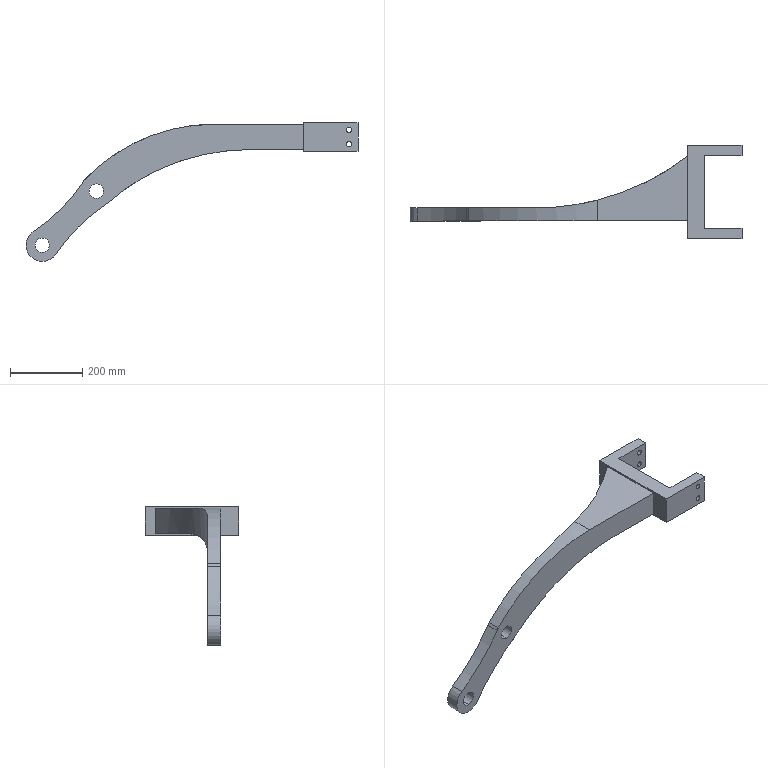Part | SolidWorks | features ICE 3, Cut 1, Extrusion 1 | 1 solid | 34 faces | box 920 x 260 x 385 mm | volume 5252996 mm3 | cylinder 20 | plane 14 | commonest cylinder face diameters 15 x8 40 x4 90 x3 1000 x2 984.464 x1 1199 x1
STEP:
#1=CARTESIAN_POINT('',(50.,-130.,-27.5));
#2=VERTEX_POINT('',#1);
#3=CARTESIAN_POINT('',(50.,-130.,-12.5));
#4=VERTEX_POINT('',#3);
#5=CARTESIAN_POINT('',(50.,-130.,-20.));
#6=DIRECTION('',(0.,1.,0.));
#7=DIRECTION('',(0.,0.,1.));
#8=AXIS2_PLACEMENT_3D('',#5,#6,#7);
#9=CIRCLE('',#8,7.5);
#10=EDGE_CURVE('',#2,#4,#9,.T.);
#11=ORIENTED_EDGE('',*,*,#10,.F.);
#12=CARTESIAN_POINT('',(50.,-100.,-27.5));
#13=VERTEX_POINT('',#12);
#14=CARTESIAN_POINT('',(50.,-130.,-27.5));
#15=DIRECTION('',(0.,1.,0.));
#16=VECTOR('',#15,1000.);
#17=LINE('',#14,#16);
#18=EDGE_CURVE('',#2,#13,#17,.T.);
#19=ORIENTED_EDGE('',*,*,#18,.T.);
#20=CARTESIAN_POINT('',(50.,-100.,-12.5));
#21=VERTEX_POINT('',#20);
#22=CARTESIAN_POINT('',(50.,-100.,-20.));
#23=DIRECTION('',(0.,-1.,0.));
#24=DIRECTION('',(0.,0.,-1.));
#25=AXIS2_PLACEMENT_3D('',#22,#23,#24);
#26=CIRCLE('',#25,7.5);
#27=EDGE_CURVE('',#21,#13,#26,.T.);
#28=ORIENTED_EDGE('',*,*,#27,.F.);
#29=CARTESIAN_POINT('',(50.,-130.,-12.5));
#30=DIRECTION('',(0.,1.,0.));
#31=VECTOR('',#30,1000.);
#32=LINE('',#29,#31);
#33=EDGE_CURVE('',#4,#21,#32,.T.);
#34=ORIENTED_EDGE('',*,*,#33,.F.);
#35=EDGE_LOOP('',(#11,#19,#28,#34));
#36=FACE_OUTER_BOUND('',#35,.T.);
#37=CARTESIAN_POINT('',(50.,-130.,-20.));
#38=DIRECTION('',(0.,1.,0.));
#39=DIRECTION('',(0.,0.,1.));
#40=AXIS2_PLACEMENT_3D('',#37,#38,#39);
#41=CYLINDRICAL_SURFACE('',#40,7.5);
#42=ADVANCED_FACE('',(#36),#41,.F.);
#43=CARTESIAN_POINT('',(50.,-130.,12.5));
#44=VERTEX_POINT('',#43);
#45=CARTESIAN_POINT('',(50.,-130.,27.5));
#46=VERTEX_POINT('',#45);
#47=CARTESIAN_POINT('',(50.,-130.,20.));
#48=DIRECTION('',(0.,1.,0.));
#49=DIRECTION('',(0.,0.,1.));
#50=AXIS2_PLACEMENT_3D('',#47,#48,#49);
#51=CIRCLE('',#50,7.5);
#52=EDGE_CURVE('',#44,#46,#51,.T.);
#53=ORIENTED_EDGE('',*,*,#52,.F.);
#54=CARTESIAN_POINT('',(50.,-100.,12.5));
#55=VERTEX_POINT('',#54);
#56=CARTESIAN_POINT('',(50.,-130.,12.5));
#57=DIRECTION('',(0.,1.,0.));
#58=VECTOR('',#57,1000.);
#59=LINE('',#56,#58);
#60=EDGE_CURVE('',#44,#55,#59,.T.);
#61=ORIENTED_EDGE('',*,*,#60,.T.);
#62=CARTESIAN_POINT('',(50.,-100.,27.5));
#63=VERTEX_POINT('',#62);
#64=CARTESIAN_POINT('',(50.,-100.,20.));
#65=DIRECTION('',(0.,-1.,0.));
#66=DIRECTION('',(0.,0.,-1.));
#67=AXIS2_PLACEMENT_3D('',#64,#65,#66);
#68=CIRCLE('',#67,7.5);
#69=EDGE_CURVE('',#63,#55,#68,.T.);
#70=ORIENTED_EDGE('',*,*,#69,.F.);
#71=CARTESIAN_POINT('',(50.,-130.,27.5));
#72=DIRECTION('',(0.,1.,0.));
#73=VECTOR('',#72,1000.);
#74=LINE('',#71,#73);
#75=EDGE_CURVE('',#46,#63,#74,.T.);
#76=ORIENTED_EDGE('',*,*,#75,.F.);
#77=EDGE_LOOP('',(#53,#61,#70,#76));
#78=FACE_OUTER_BOUND('',#77,.T.);
#79=CARTESIAN_POINT('',(50.,-130.,20.));
#80=DIRECTION('',(0.,1.,0.));
#81=DIRECTION('',(0.,0.,1.));
#82=AXIS2_PLACEMENT_3D('',#79,#80,#81);
#83=CYLINDRICAL_SURFACE('',#82,7.5);
#84=ADVANCED_FACE('',(#78),#83,.F.);
#85=CARTESIAN_POINT('',(50.,100.,-27.5));
#86=VERTEX_POINT('',#85);
#87=CARTESIAN_POINT('',(50.,100.,-12.5));
#88=VERTEX_POINT('',#87);
#89=CARTESIAN_POINT('',(50.,100.,-20.));
#90=DIRECTION('',(0.,1.,0.));
#91=DIRECTION('',(0.,0.,1.));
#92=AXIS2_PLACEMENT_3D('',#89,#90,#91);
#93=CIRCLE('',#92,7.5);
#94=EDGE_CURVE('',#86,#88,#93,.T.);
#95=ORIENTED_EDGE('',*,*,#94,.F.);
#96=CARTESIAN_POINT('',(50.,130.,-27.5));
#97=VERTEX_POINT('',#96);
#98=CARTESIAN_POINT('',(50.,-130.,-27.5));
#99=DIRECTION('',(0.,1.,0.));
#100=VECTOR('',#99,1000.);
#101=LINE('',#98,#100);
#102=EDGE_CURVE('',#86,#97,#101,.T.);
#103=ORIENTED_EDGE('',*,*,#102,.T.);
#104=CARTESIAN_POINT('',(50.,130.,-12.5));
#105=VERTEX_POINT('',#104);
#106=CARTESIAN_POINT('',(50.,130.,-20.));
#107=DIRECTION('',(0.,1.,0.));
#108=DIRECTION('',(0.,0.,1.));
#109=AXIS2_PLACEMENT_3D('',#106,#107,#108);
#110=CIRCLE('',#109,7.5);
#111=EDGE_CURVE('',#97,#105,#110,.T.);
#112=ORIENTED_EDGE('',*,*,#111,.T.);
#113=CARTESIAN_POINT('',(50.,-130.,-12.5));
#114=DIRECTION('',(0.,1.,0.));
#115=VECTOR('',#114,1000.);
#116=LINE('',#113,#115);
#117=EDGE_CURVE('',#88,#105,#116,.T.);
#118=ORIENTED_EDGE('',*,*,#117,.F.);
#119=EDGE_LOOP('',(#95,#103,#112,#118));
#120=FACE_OUTER_BOUND('',#119,.T.);
#121=CARTESIAN_POINT('',(50.,-130.,-20.));
#122=DIRECTION('',(0.,1.,0.));
#123=DIRECTION('',(0.,0.,1.));
#124=AXIS2_PLACEMENT_3D('',#121,#122,#123);
#125=CYLINDRICAL_SURFACE('',#124,7.5);
#126=ADVANCED_FACE('',(#120),#125,.F.);
#127=CARTESIAN_POINT('',(50.,100.,12.5));
#128=VERTEX_POINT('',#127);
#129=CARTESIAN_POINT('',(50.,100.,27.5));
#130=VERTEX_POINT('',#129);
#131=CARTESIAN_POINT('',(50.,100.,20.));
#132=DIRECTION('',(0.,1.,0.));
#133=DIRECTION('',(0.,0.,1.));
#134=AXIS2_PLACEMENT_3D('',#131,#132,#133);
#135=CIRCLE('',#134,7.5);
#136=EDGE_CURVE('',#128,#130,#135,.T.);
#137=ORIENTED_EDGE('',*,*,#136,.F.);
#138=CARTESIAN_POINT('',(50.,130.,12.5));
#139=VERTEX_POINT('',#138);
#140=CARTESIAN_POINT('',(50.,-130.,12.5));
#141=DIRECTION('',(0.,1.,0.));
#142=VECTOR('',#141,1000.);
#143=LINE('',#140,#142);
#144=EDGE_CURVE('',#128,#139,#143,.T.);
#145=ORIENTED_EDGE('',*,*,#144,.T.);
#146=CARTESIAN_POINT('',(50.,130.,27.5));
#147=VERTEX_POINT('',#146);
#148=CARTESIAN_POINT('',(50.,130.,20.));
#149=DIRECTION('',(0.,1.,0.));
#150=DIRECTION('',(0.,0.,1.));
#151=AXIS2_PLACEMENT_3D('',#148,#149,#150);
#152=CIRCLE('',#151,7.5);
#153=EDGE_CURVE('',#139,#147,#152,.T.);
#154=ORIENTED_EDGE('',*,*,#153,.T.);
#155=CARTESIAN_POINT('',(50.,-130.,27.5));
#156=DIRECTION('',(0.,1.,0.));
#157=VECTOR('',#156,1000.);
#158=LINE('',#155,#157);
#159=EDGE_CURVE('',#130,#147,#158,.T.);
#160=ORIENTED_EDGE('',*,*,#159,.F.);
#161=EDGE_LOOP('',(#137,#145,#154,#160));
#162=FACE_OUTER_BOUND('',#161,.T.);
#163=CARTESIAN_POINT('',(50.,-130.,20.));
#164=DIRECTION('',(0.,1.,0.));
#165=DIRECTION('',(0.,0.,1.));
#166=AXIS2_PLACEMENT_3D('',#163,#164,#165);
#167=CYLINDRICAL_SURFACE('',#166,7.5);
#168=ADVANCED_FACE('',(#162),#167,.F.);
#169=CARTESIAN_POINT('',(-650.,-80.,-130.));
#170=VERTEX_POINT('',#169);
#171=CARTESIAN_POINT('',(-650.,-80.,-170.));
#172=VERTEX_POINT('',#171);
#173=CARTESIAN_POINT('',(-650.,-80.,-150.));
#174=DIRECTION('',(0.,-1.,0.));
#175=DIRECTION('',(-1.,0.,0.));
#176=AXIS2_PLACEMENT_3D('',#173,#174,#175);
#177=CIRCLE('',#176,20.);
#178=EDGE_CURVE('',#170,#172,#177,.T.);
#179=ORIENTED_EDGE('',*,*,#178,.T.);
#180=CARTESIAN_POINT('',(-650.,-43.779,-170.));
#181=VERTEX_POINT('',#180);
#182=CARTESIAN_POINT('',(-650.,-100.,-170.));
#183=DIRECTION('',(0.,1.,0.));
#184=VECTOR('',#183,1000.);
#185=LINE('',#182,#184);
#186=EDGE_CURVE('',#172,#181,#185,.T.);
#187=ORIENTED_EDGE('',*,*,#186,.T.);
#188=CARTESIAN_POINT('',(-650.,-43.779,-130.));
#189=VERTEX_POINT('',#188);
#190=CARTESIAN_POINT('',(-650.,-43.779,-150.));
#191=DIRECTION('',(0.,1.,0.));
#192=DIRECTION('',(0.,0.,-1.));
#193=AXIS2_PLACEMENT_3D('',#190,#191,#192);
#194=CIRCLE('',#193,20.);
#195=EDGE_CURVE('',#181,#189,#194,.T.);
#196=ORIENTED_EDGE('',*,*,#195,.T.);
#197=CARTESIAN_POINT('',(-650.,-100.,-130.));
#198=DIRECTION('',(0.,1.,0.));
#199=VECTOR('',#198,1000.);
#200=LINE('',#197,#199);
#201=EDGE_CURVE('',#170,#189,#200,.T.);
#202=ORIENTED_EDGE('',*,*,#201,.F.);
#203=EDGE_LOOP('',(#179,#187,#196,#202));
#204=FACE_OUTER_BOUND('',#203,.T.);
#205=CARTESIAN_POINT('',(-650.,-100.,-150.));
#206=DIRECTION('',(0.,1.,0.));
#207=DIRECTION('',(0.,0.,1.));
#208=AXIS2_PLACEMENT_3D('',#205,#206,#207);
#209=CYLINDRICAL_SURFACE('',#208,20.);
#210=ADVANCED_FACE('',(#204),#209,.F.);
#211=CARTESIAN_POINT('',(-800.,-80.,-280.));
#212=VERTEX_POINT('',#211);
#213=CARTESIAN_POINT('',(-800.,-80.,-320.));
#214=VERTEX_POINT('',#213);
#215=CARTESIAN_POINT('',(-800.,-80.,-300.));
#216=DIRECTION('',(0.,-1.,0.));
#217=DIRECTION('',(-1.,0.,0.));
#218=AXIS2_PLACEMENT_3D('',#215,#216,#217);
#219=CIRCLE('',#218,20.);
#220=EDGE_CURVE('',#212,#214,#219,.T.);
#221=ORIENTED_EDGE('',*,*,#220,.T.);
#222=CARTESIAN_POINT('',(-800.,-43.779,-320.));
#223=VERTEX_POINT('',#222);
#224=CARTESIAN_POINT('',(-800.,-100.,-320.));
#225=DIRECTION('',(0.,1.,0.));
#226=VECTOR('',#225,1000.);
#227=LINE('',#224,#226);
#228=EDGE_CURVE('',#214,#223,#227,.T.);
#229=ORIENTED_EDGE('',*,*,#228,.T.);
#230=CARTESIAN_POINT('',(-800.,-43.779,-280.));
#231=VERTEX_POINT('',#230);
#232=CARTESIAN_POINT('',(-800.,-43.779,-300.));
#233=DIRECTION('',(0.,1.,0.));
#234=DIRECTION('',(0.,0.,-1.));
#235=AXIS2_PLACEMENT_3D('',#232,#233,#234);
#236=CIRCLE('',#235,20.);
#237=EDGE_CURVE('',#223,#231,#236,.T.);
#238=ORIENTED_EDGE('',*,*,#237,.T.);
#239=CARTESIAN_POINT('',(-800.,-100.,-280.));
#240=DIRECTION('',(0.,1.,0.));
#241=VECTOR('',#240,1000.);
#242=LINE('',#239,#241);
#243=EDGE_CURVE('',#212,#231,#242,.T.);
#244=ORIENTED_EDGE('',*,*,#243,.F.);
#245=EDGE_LOOP('',(#221,#229,#238,#244));
#246=FACE_OUTER_BOUND('',#245,.T.);
#247=CARTESIAN_POINT('',(-800.,-100.,-300.));
#248=DIRECTION('',(0.,1.,0.));
#249=DIRECTION('',(0.,0.,1.));
#250=AXIS2_PLACEMENT_3D('',#247,#248,#249);
#251=CYLINDRICAL_SURFACE('',#250,20.);
#252=ADVANCED_FACE('',(#246),#251,.F.);
#253=CARTESIAN_POINT('',(-75.,100.,35.));
#254=VERTEX_POINT('',#253);
#255=CARTESIAN_POINT('',(-75.,100.,-35.));
#256=VERTEX_POINT('',#255);
#257=CARTESIAN_POINT('',(-75.,100.,-35.));
#258=DIRECTION('',(0.,0.,-1.));
#259=VECTOR('',#258,1000.);
#260=LINE('',#257,#259);
#261=EDGE_CURVE('',#254,#256,#260,.T.);
#262=ORIENTED_EDGE('',*,*,#261,.F.);
#263=CARTESIAN_POINT('',(-75.,-80.,35.));
#264=VERTEX_POINT('',#263);
#265=CARTESIAN_POINT('',(-75.,-100.,35.));
#266=DIRECTION('',(0.,1.,0.));
#267=VECTOR('',#266,1000.);
#268=LINE('',#265,#267);
#269=EDGE_CURVE('',#264,#254,#268,.T.);
#270=ORIENTED_EDGE('',*,*,#269,.F.);
#271=CARTESIAN_POINT('',(-75.,-80.,-35.));
#272=VERTEX_POINT('',#271);
#273=CARTESIAN_POINT('',(-75.,-80.,-345.));
#274=DIRECTION('',(0.,0.,1.));
#275=VECTOR('',#274,1000.);
#276=LINE('',#273,#275);
#277=EDGE_CURVE('',#272,#264,#276,.T.);
#278=ORIENTED_EDGE('',*,*,#277,.F.);
#279=CARTESIAN_POINT('',(-75.,-100.,-35.));
#280=DIRECTION('',(0.,1.,0.));
#281=VECTOR('',#280,1000.);
#282=LINE('',#279,#281);
#283=EDGE_CURVE('',#272,#256,#282,.T.);
#284=ORIENTED_EDGE('',*,*,#283,.T.);
#285=EDGE_LOOP('',(#262,#270,#278,#284));
#286=FACE_BOUND('',#285,.T.);
#287=CARTESIAN_POINT('',(-75.,130.,-40.));
#288=VERTEX_POINT('',#287);
#289=CARTESIAN_POINT('',(-75.,-130.,-40.));
#290=VERTEX_POINT('',#289);
#291=CARTESIAN_POINT('',(-75.,130.,-40.));
#292=DIRECTION('',(0.,-1.,0.));
#293=VECTOR('',#292,1000.);
#294=LINE('',#291,#293);
#295=EDGE_CURVE('',#288,#290,#294,.T.);
#296=ORIENTED_EDGE('',*,*,#295,.T.);
#297=CARTESIAN_POINT('',(-75.,-130.,40.));
#298=VERTEX_POINT('',#297);
#299=CARTESIAN_POINT('',(-75.,-130.,40.));
#300=DIRECTION('',(0.,0.,-1.));
#301=VECTOR('',#300,1000.);
#302=LINE('',#299,#301);
#303=EDGE_CURVE('',#298,#290,#302,.T.);
#304=ORIENTED_EDGE('',*,*,#303,.F.);
#305=CARTESIAN_POINT('',(-75.,130.,40.));
#306=VERTEX_POINT('',#305);
#307=CARTESIAN_POINT('',(-75.,130.,40.));
#308=DIRECTION('',(0.,-1.,0.));
#309=VECTOR('',#308,1000.);
#310=LINE('',#307,#309);
#311=EDGE_CURVE('',#306,#298,#310,.T.);
#312=ORIENTED_EDGE('',*,*,#311,.F.);
#313=CARTESIAN_POINT('',(-75.,130.,40.));
#314=DIRECTION('',(0.,0.,-1.));
#315=VECTOR('',#314,1000.);
#316=LINE('',#313,#315);
#317=EDGE_CURVE('',#306,#288,#316,.T.);
#318=ORIENTED_EDGE('',*,*,#317,.T.);
#319=EDGE_LOOP('',(#296,#304,#312,#318));
#320=FACE_OUTER_BOUND('',#319,.T.);
#321=CARTESIAN_POINT('',(-75.,130.,40.));
#322=DIRECTION('',(1.,0.,0.));
#323=DIRECTION('',(0.,1.,0.));
#324=AXIS2_PLACEMENT_3D('',#321,#322,#323);
#325=PLANE('',#324);
#326=ADVANCED_FACE('',(#286,#320),#325,.F.);
#327=CARTESIAN_POINT('',(75.,-130.,-40.));
#328=VERTEX_POINT('',#327);
#329=CARTESIAN_POINT('',(75.,-100.,-40.));
#330=VERTEX_POINT('',#329);
#331=CARTESIAN_POINT('',(75.,130.,-40.));
#332=DIRECTION('',(0.,1.,0.));
#333=VECTOR('',#332,1000.);
#334=LINE('',#331,#333);
#335=EDGE_CURVE('',#328,#330,#334,.T.);
#336=ORIENTED_EDGE('',*,*,#335,.T.);
#337=CARTESIAN_POINT('',(75.,-100.,40.));
#338=VERTEX_POINT('',#337);
#339=CARTESIAN_POINT('',(75.,-100.,40.));
#340=DIRECTION('',(0.,0.,1.));
#341=VECTOR('',#340,1000.);
#342=LINE('',#339,#341);
#343=EDGE_CURVE('',#330,#338,#342,.T.);
#344=ORIENTED_EDGE('',*,*,#343,.T.);
#345=CARTESIAN_POINT('',(75.,-130.,40.));
#346=VERTEX_POINT('',#345);
#347=CARTESIAN_POINT('',(75.,130.,40.));
#348=DIRECTION('',(0.,1.,0.));
#349=VECTOR('',#348,1000.);
#350=LINE('',#347,#349);
#351=EDGE_CURVE('',#346,#338,#350,.T.);
#352=ORIENTED_EDGE('',*,*,#351,.F.);
#353=CARTESIAN_POINT('',(75.,-130.,40.));
#354=DIRECTION('',(0.,0.,-1.));
#355=VECTOR('',#354,1000.);
#356=LINE('',#353,#355);
#357=EDGE_CURVE('',#346,#328,#356,.T.);
#358=ORIENTED_EDGE('',*,*,#357,.T.);
#359=EDGE_LOOP('',(#336,#344,#352,#358));
#360=FACE_OUTER_BOUND('',#359,.T.);
#361=CARTESIAN_POINT('',(75.,130.,40.));
#362=DIRECTION('',(-1.,0.,0.));
#363=DIRECTION('',(0.,-1.,0.));
#364=AXIS2_PLACEMENT_3D('',#361,#362,#363);
#365=PLANE('',#364);
#366=ADVANCED_FACE('',(#360),#365,.F.);
#367=CARTESIAN_POINT('',(75.,100.,40.));
#368=VERTEX_POINT('',#367);
#369=CARTESIAN_POINT('',(75.,130.,40.));
#370=VERTEX_POINT('',#369);
#371=CARTESIAN_POINT('',(75.,130.,40.));
#372=DIRECTION('',(0.,1.,0.));
#373=VECTOR('',#372,1000.);
#374=LINE('',#371,#373);
#375=EDGE_CURVE('',#368,#370,#374,.T.);
#376=ORIENTED_EDGE('',*,*,#375,.F.);
#377=CARTESIAN_POINT('',(75.,100.,-40.));
#378=VERTEX_POINT('',#377);
#379=CARTESIAN_POINT('',(75.,100.,40.));
#380=DIRECTION('',(0.,0.,-1.));
#381=VECTOR('',#380,1000.);
#382=LINE('',#379,#381);
#383=EDGE_CURVE('',#368,#378,#382,.T.);
#384=ORIENTED_EDGE('',*,*,#383,.T.);
#385=CARTESIAN_POINT('',(75.,130.,-40.));
#386=VERTEX_POINT('',#385);
#387=CARTESIAN_POINT('',(75.,130.,-40.));
#388=DIRECTION('',(0.,1.,0.));
#389=VECTOR('',#388,1000.);
#390=LINE('',#387,#389);
#391=EDGE_CURVE('',#378,#386,#390,.T.);
#392=ORIENTED_EDGE('',*,*,#391,.T.);
#393=CARTESIAN_POINT('',(75.,130.,40.));
#394=DIRECTION('',(0.,0.,-1.));
#395=VECTOR('',#394,1000.);
#396=LINE('',#393,#395);
#397=EDGE_CURVE('',#370,#386,#396,.T.);
#398=ORIENTED_EDGE('',*,*,#397,.F.);
#399=EDGE_LOOP('',(#376,#384,#392,#398));
#400=FACE_OUTER_BOUND('',#399,.T.);
#401=CARTESIAN_POINT('',(75.,130.,40.));
#402=DIRECTION('',(-1.,0.,0.));
#403=DIRECTION('',(0.,-1.,0.));
#404=AXIS2_PLACEMENT_3D('',#401,#402,#403);
#405=PLANE('',#404);
#406=ADVANCED_FACE('',(#400),#405,.F.);
#407=CARTESIAN_POINT('',(50.,130.,-20.));
#408=DIRECTION('',(0.,1.,0.));
#409=DIRECTION('',(0.,0.,1.));
#410=AXIS2_PLACEMENT_3D('',#407,#408,#409);
#411=CIRCLE('',#410,7.5);
#412=EDGE_CURVE('',#105,#97,#411,.T.);
#413=ORIENTED_EDGE('',*,*,#412,.F.);
#414=ORIENTED_EDGE('',*,*,#111,.F.);
#415=EDGE_LOOP('',(#413,#414));
#416=FACE_BOUND('',#415,.T.);
#417=CARTESIAN_POINT('',(50.,130.,20.));
#418=DIRECTION('',(0.,1.,0.));
#419=DIRECTION('',(0.,0.,1.));
#420=AXIS2_PLACEMENT_3D('',#417,#418,#419);
#421=CIRCLE('',#420,7.5);
#422=EDGE_CURVE('',#147,#139,#421,.T.);
#423=ORIENTED_EDGE('',*,*,#422,.F.);
#424=ORIENTED_EDGE('',*,*,#153,.F.);
#425=EDGE_LOOP('',(#423,#424));
#426=FACE_BOUND('',#425,.T.);
#427=CARTESIAN_POINT('',(-75.,130.,-40.));
#428=DIRECTION('',(-1.,0.,0.));
#429=VECTOR('',#428,1000.);
#430=LINE('',#427,#429);
#431=EDGE_CURVE('',#386,#288,#430,.T.);
#432=ORIENTED_EDGE('',*,*,#431,.T.);
#433=ORIENTED_EDGE('',*,*,#317,.F.);
#434=CARTESIAN_POINT('',(-75.,130.,40.));
#435=DIRECTION('',(-1.,0.,0.));
#436=VECTOR('',#435,1000.);
#437=LINE('',#434,#436);
#438=EDGE_CURVE('',#370,#306,#437,.T.);
#439=ORIENTED_EDGE('',*,*,#438,.F.);
#440=ORIENTED_EDGE('',*,*,#397,.T.);
#441=EDGE_LOOP('',(#432,#433,#439,#440));
#442=FACE_OUTER_BOUND('',#441,.T.);
#443=CARTESIAN_POINT('',(-75.,130.,40.));
#444=DIRECTION('',(0.,-1.,0.));
#445=DIRECTION('',(0.,0.,-1.));
#446=AXIS2_PLACEMENT_3D('',#443,#444,#445);
#447=PLANE('',#446);
#448=ADVANCED_FACE('',(#416,#426,#442),#447,.F.);
#449=CARTESIAN_POINT('',(50.,-130.,-20.));
#450=DIRECTION('',(0.,1.,0.));
#451=DIRECTION('',(0.,0.,1.));
#452=AXIS2_PLACEMENT_3D('',#449,#450,#451);
#453=CIRCLE('',#452,7.5);
#454=EDGE_CURVE('',#4,#2,#453,.T.);
#455=ORIENTED_EDGE('',*,*,#454,.T.);
#456=ORIENTED_EDGE('',*,*,#10,.T.);
#457=EDGE_LOOP('',(#455,#456));
#458=FACE_BOUND('',#457,.T.);
#459=CARTESIAN_POINT('',(50.,-130.,20.));
#460=DIRECTION('',(0.,1.,0.));
#461=DIRECTION('',(0.,0.,1.));
#462=AXIS2_PLACEMENT_3D('',#459,#460,#461);
#463=CIRCLE('',#462,7.5);
#464=EDGE_CURVE('',#46,#44,#463,.T.);
#465=ORIENTED_EDGE('',*,*,#464,.T.);
#466=ORIENTED_EDGE('',*,*,#52,.T.);
#467=EDGE_LOOP('',(#465,#466));
#468=FACE_BOUND('',#467,.T.);
#469=CARTESIAN_POINT('',(-75.,-130.,-40.));
#470=DIRECTION('',(1.,0.,0.));
#471=VECTOR('',#470,1000.);
#472=LINE('',#469,#471);
#473=EDGE_CURVE('',#290,#328,#472,.T.);
#474=ORIENTED_EDGE('',*,*,#473,.T.);
#475=ORIENTED_EDGE('',*,*,#357,.F.);
#476=CARTESIAN_POINT('',(-75.,-130.,40.));
#477=DIRECTION('',(1.,0.,0.));
#478=VECTOR('',#477,1000.);
#479=LINE('',#476,#478);
#480=EDGE_CURVE('',#298,#346,#479,.T.);
#481=ORIENTED_EDGE('',*,*,#480,.F.);
#482=ORIENTED_EDGE('',*,*,#303,.T.);
#483=EDGE_LOOP('',(#474,#475,#481,#482));
#484=FACE_OUTER_BOUND('',#483,.T.);
#485=CARTESIAN_POINT('',(-75.,-130.,40.));
#486=DIRECTION('',(0.,1.,0.));
#487=DIRECTION('',(0.,0.,1.));
#488=AXIS2_PLACEMENT_3D('',#485,#486,#487);
#489=PLANE('',#488);
#490=ADVANCED_FACE('',(#458,#468,#484),#489,.F.);
#491=CARTESIAN_POINT('',(-30.,-100.,40.));
#492=VERTEX_POINT('',#491);
#493=CARTESIAN_POINT('',(-30.,-100.,40.));
#494=DIRECTION('',(1.,0.,0.));
#495=VECTOR('',#494,1000.);
#496=LINE('',#493,#495);
#497=EDGE_CURVE('',#492,#338,#496,.T.);
#498=ORIENTED_EDGE('',*,*,#497,.F.);
#499=CARTESIAN_POINT('',(-30.,100.,40.));
#500=VERTEX_POINT('',#499);
#501=CARTESIAN_POINT('',(-30.,100.,40.));
#502=DIRECTION('',(0.,-1.,0.));
#503=VECTOR('',#502,1000.);
#504=LINE('',#501,#503);
#505=EDGE_CURVE('',#500,#492,#504,.T.);
#506=ORIENTED_EDGE('',*,*,#505,.F.);
#507=CARTESIAN_POINT('',(-30.,100.,40.));
#508=DIRECTION('',(-1.,0.,0.));
#509=VECTOR('',#508,1000.);
#510=LINE('',#507,#509);
#511=EDGE_CURVE('',#368,#500,#510,.T.);
#512=ORIENTED_EDGE('',*,*,#511,.F.);
#513=ORIENTED_EDGE('',*,*,#375,.T.);
#514=ORIENTED_EDGE('',*,*,#438,.T.);
#515=ORIENTED_EDGE('',*,*,#311,.T.);
#516=ORIENTED_EDGE('',*,*,#480,.T.);
#517=ORIENTED_EDGE('',*,*,#351,.T.);
#518=EDGE_LOOP('',(#498,#506,#512,#513,#514,#515,#516,#517));
#519=FACE_OUTER_BOUND('',#518,.T.);
#520=CARTESIAN_POINT('',(0.,0.,40.));
#521=DIRECTION('',(0.,0.,1.));
#522=DIRECTION('',(1.,0.,0.));
#523=AXIS2_PLACEMENT_3D('',#520,#521,#522);
#524=PLANE('',#523);
#525=ADVANCED_FACE('',(#519),#524,.T.);
#526=CARTESIAN_POINT('',(-30.,100.,-40.));
#527=VERTEX_POINT('',#526);
#528=CARTESIAN_POINT('',(-30.,-100.,-40.));
#529=VERTEX_POINT('',#528);
#530=CARTESIAN_POINT('',(-30.,100.,-40.));
#531=DIRECTION('',(0.,-1.,0.));
#532=VECTOR('',#531,1000.);
#533=LINE('',#530,#532);
#534=EDGE_CURVE('',#527,#529,#533,.T.);
#535=ORIENTED_EDGE('',*,*,#534,.T.);
#536=CARTESIAN_POINT('',(-30.,-100.,-40.));
#537=DIRECTION('',(1.,0.,0.));
#538=VECTOR('',#537,1000.);
#539=LINE('',#536,#538);
#540=EDGE_CURVE('',#529,#330,#539,.T.);
#541=ORIENTED_EDGE('',*,*,#540,.T.);
#542=ORIENTED_EDGE('',*,*,#335,.F.);
#543=ORIENTED_EDGE('',*,*,#473,.F.);
#544=ORIENTED_EDGE('',*,*,#295,.F.);
#545=ORIENTED_EDGE('',*,*,#431,.F.);
#546=ORIENTED_EDGE('',*,*,#391,.F.);
#547=CARTESIAN_POINT('',(0.,100.,-40.));
#548=DIRECTION('',(-1.,0.,0.));
#549=VECTOR('',#548,1000.);
#550=LINE('',#547,#549);
#551=EDGE_CURVE('',#378,#527,#550,.T.);
#552=ORIENTED_EDGE('',*,*,#551,.T.);
#553=EDGE_LOOP('',(#535,#541,#542,#543,#544,#545,#546,#552));
#554=FACE_OUTER_BOUND('',#553,.T.);
#555=CARTESIAN_POINT('',(0.,0.,-40.));
#556=DIRECTION('',(0.,0.,1.));
#557=DIRECTION('',(1.,0.,0.));
#558=AXIS2_PLACEMENT_3D('',#555,#556,#557);
#559=PLANE('',#558);
#560=ADVANCED_FACE('',(#554),#559,.F.);
#561=ORIENTED_EDGE('',*,*,#27,.T.);
#562=CARTESIAN_POINT('',(50.,-100.,-20.));
#563=DIRECTION('',(0.,-1.,0.));
#564=DIRECTION('',(0.,0.,-1.));
#565=AXIS2_PLACEMENT_3D('',#562,#563,#564);
#566=CIRCLE('',#565,7.5);
#567=EDGE_CURVE('',#13,#21,#566,.T.);
#568=ORIENTED_EDGE('',*,*,#567,.T.);
#569=EDGE_LOOP('',(#561,#568));
#570=FACE_BOUND('',#569,.T.);
#571=ORIENTED_EDGE('',*,*,#69,.T.);
#572=CARTESIAN_POINT('',(50.,-100.,20.));
#573=DIRECTION('',(0.,-1.,0.));
#574=DIRECTION('',(0.,0.,-1.));
#575=AXIS2_PLACEMENT_3D('',#572,#573,#574);
#576=CIRCLE('',#575,7.5);
#577=EDGE_CURVE('',#55,#63,#576,.T.);
#578=ORIENTED_EDGE('',*,*,#577,.T.);
#579=EDGE_LOOP('',(#571,#578));
#580=FACE_BOUND('',#579,.T.);
#581=ORIENTED_EDGE('',*,*,#540,.F.);
#582=CARTESIAN_POINT('',(-30.,-100.,-40.));
#583=DIRECTION('',(0.,0.,1.));
#584=VECTOR('',#583,1000.);
#585=LINE('',#582,#584);
#586=EDGE_CURVE('',#529,#492,#585,.T.);
#587=ORIENTED_EDGE('',*,*,#586,.T.);
#588=ORIENTED_EDGE('',*,*,#497,.T.);
#589=ORIENTED_EDGE('',*,*,#343,.F.);
#590=EDGE_LOOP('',(#581,#587,#588,#589));
#591=FACE_OUTER_BOUND('',#590,.T.);
#592=CARTESIAN_POINT('',(-30.,-100.,-40.));
#593=DIRECTION('',(0.,-1.,0.));
#594=DIRECTION('',(0.,0.,-1.));
#595=AXIS2_PLACEMENT_3D('',#592,#593,#594);
#596=PLANE('',#595);
#597=ADVANCED_FACE('',(#570,#580,#591),#596,.F.);
#598=CARTESIAN_POINT('',(50.,100.,-20.));
#599=DIRECTION('',(0.,1.,0.));
#600=DIRECTION('',(0.,0.,1.));
#601=AXIS2_PLACEMENT_3D('',#598,#599,#600);
#602=CIRCLE('',#601,7.5);
#603=EDGE_CURVE('',#88,#86,#602,.T.);
#604=ORIENTED_EDGE('',*,*,#603,.T.);
#605=ORIENTED_EDGE('',*,*,#94,.T.);
#606=EDGE_LOOP('',(#604,#605));
#607=FACE_BOUND('',#606,.T.);
#608=CARTESIAN_POINT('',(50.,100.,20.));
#609=DIRECTION('',(0.,1.,0.));
#610=DIRECTION('',(0.,0.,1.));
#611=AXIS2_PLACEMENT_3D('',#608,#609,#610);
#612=CIRCLE('',#611,7.5);
#613=EDGE_CURVE('',#130,#128,#612,.T.);
#614=ORIENTED_EDGE('',*,*,#613,.T.);
#615=ORIENTED_EDGE('',*,*,#136,.T.);
#616=EDGE_LOOP('',(#614,#615));
#617=FACE_BOUND('',#616,.T.);
#618=ORIENTED_EDGE('',*,*,#511,.T.);
#619=CARTESIAN_POINT('',(-30.,100.,-40.));
#620=DIRECTION('',(0.,0.,1.));
#621=VECTOR('',#620,1000.);
#622=LINE('',#619,#621);
#623=EDGE_CURVE('',#527,#500,#622,.T.);
#624=ORIENTED_EDGE('',*,*,#623,.F.);
#625=ORIENTED_EDGE('',*,*,#551,.F.);
#626=ORIENTED_EDGE('',*,*,#383,.F.);
#627=EDGE_LOOP('',(#618,#624,#625,#626));
#628=FACE_OUTER_BOUND('',#627,.T.);
#629=CARTESIAN_POINT('',(-30.,100.,-40.));
#630=DIRECTION('',(0.,1.,0.));
#631=DIRECTION('',(0.,0.,1.));
#632=AXIS2_PLACEMENT_3D('',#629,#630,#631);
#633=PLANE('',#632);
#634=ADVANCED_FACE('',(#607,#617,#628),#633,.F.);
#635=ORIENTED_EDGE('',*,*,#505,.T.);
#636=ORIENTED_EDGE('',*,*,#586,.F.);
#637=ORIENTED_EDGE('',*,*,#534,.F.);
#638=ORIENTED_EDGE('',*,*,#623,.T.);
#639=EDGE_LOOP('',(#635,#636,#637,#638));
#640=FACE_OUTER_BOUND('',#639,.T.);
#641=CARTESIAN_POINT('',(-30.,100.,-40.));
#642=DIRECTION('',(-1.,0.,0.));
#643=DIRECTION('',(0.,-1.,0.));
#644=AXIS2_PLACEMENT_3D('',#641,#642,#643);
#645=PLANE('',#644);
#646=ADVANCED_FACE('',(#640),#645,.F.);
#647=CARTESIAN_POINT('',(-225.,11.648,-35.));
#648=VERTEX_POINT('',#647);
#649=CARTESIAN_POINT('',(-495.,641.552,-35.));
#650=DIRECTION('',(0.,0.,-1.));
#651=DIRECTION('',(-1.,0.,0.));
#652=AXIS2_PLACEMENT_3D('',#649,#650,#651);
#653=CIRCLE('',#652,685.331);
#654=EDGE_CURVE('',#256,#648,#653,.T.);
#655=ORIENTED_EDGE('',*,*,#654,.F.);
#656=ORIENTED_EDGE('',*,*,#283,.F.);
#657=CARTESIAN_POINT('',(-225.,-80.,-35.));
#658=VERTEX_POINT('',#657);
#659=CARTESIAN_POINT('',(-75.,-80.,-35.));
#660=DIRECTION('',(1.,0.,0.));
#661=VECTOR('',#660,1000.);
#662=LINE('',#659,#661);
#663=EDGE_CURVE('',#658,#272,#662,.T.);
#664=ORIENTED_EDGE('',*,*,#663,.F.);
#665=CARTESIAN_POINT('',(-225.,-100.,-35.));
#666=DIRECTION('',(0.,1.,0.));
#667=VECTOR('',#666,1000.);
#668=LINE('',#665,#667);
#669=EDGE_CURVE('',#658,#648,#668,.T.);
#670=ORIENTED_EDGE('',*,*,#669,.T.);
#671=EDGE_LOOP('',(#655,#656,#664,#670));
#672=FACE_OUTER_BOUND('',#671,.T.);
#673=CARTESIAN_POINT('',(-75.,-100.,-35.));
#674=DIRECTION('',(0.,0.,-1.));
#675=DIRECTION('',(-1.,0.,0.));
#676=AXIS2_PLACEMENT_3D('',#673,#674,#675);
#677=PLANE('',#676);
#678=ADVANCED_FACE('',(#672),#677,.T.);
#679=CARTESIAN_POINT('',(-325.,-22.36,35.));
#680=VERTEX_POINT('',#679);
#681=CARTESIAN_POINT('',(-495.,641.552,35.));
#682=DIRECTION('',(0.,0.,1.));
#683=DIRECTION('',(1.,0.,0.));
#684=AXIS2_PLACEMENT_3D('',#681,#682,#683);
#685=CIRCLE('',#684,685.331);
#686=EDGE_CURVE('',#680,#254,#685,.T.);
#687=ORIENTED_EDGE('',*,*,#686,.F.);
#688=CARTESIAN_POINT('',(-325.,-80.,35.));
#689=VERTEX_POINT('',#688);
#690=CARTESIAN_POINT('',(-325.,-100.,35.));
#691=DIRECTION('',(0.,1.,0.));
#692=VECTOR('',#691,1000.);
#693=LINE('',#690,#692);
#694=EDGE_CURVE('',#689,#680,#693,.T.);
#695=ORIENTED_EDGE('',*,*,#694,.F.);
#696=CARTESIAN_POINT('',(-75.,-80.,35.));
#697=DIRECTION('',(-1.,0.,0.));
#698=VECTOR('',#697,1000.);
#699=LINE('',#696,#698);
#700=EDGE_CURVE('',#264,#689,#699,.T.);
#701=ORIENTED_EDGE('',*,*,#700,.F.);
#702=ORIENTED_EDGE('',*,*,#269,.T.);
#703=EDGE_LOOP('',(#687,#695,#701,#702));
#704=FACE_OUTER_BOUND('',#703,.T.);
#705=CARTESIAN_POINT('',(-75.,-100.,35.));
#706=DIRECTION('',(0.,0.,1.));
#707=DIRECTION('',(1.,0.,0.));
#708=AXIS2_PLACEMENT_3D('',#705,#706,#707);
#709=PLANE('',#708);
#710=ADVANCED_FACE('',(#704),#709,.T.);
#711=CARTESIAN_POINT('',(-495.,-43.779,4.712));
#712=VERTEX_POINT('',#711);
#713=CARTESIAN_POINT('',(-495.,-43.779,4.712));
#714=CARTESIAN_POINT('',(-481.417,-43.779,9.711));
#715=CARTESIAN_POINT('',(-467.617,-43.376,14.11));
#716=CARTESIAN_POINT('',(-446.59,-42.103,19.801));
#717=CARTESIAN_POINT('',(-439.527,-41.568,21.547));
#718=CARTESIAN_POINT('',(-428.848,-40.588,23.935));
#719=CARTESIAN_POINT('',(-425.275,-40.232,24.692));
#720=CARTESIAN_POINT('',(-419.894,-39.654,25.77));
#721=CARTESIAN_POINT('',(-418.096,-39.453,26.12));
#722=CARTESIAN_POINT('',(-414.504,-39.038,26.798));
#723=CARTESIAN_POINT('',(-412.708,-38.823,27.126));
#724=CARTESIAN_POINT('',(-396.549,-36.825,29.991));
#725=CARTESIAN_POINT('',(-382.205,-34.59,31.876));
#726=CARTESIAN_POINT('',(-353.564,-29.184,34.381));
#727=CARTESIAN_POINT('',(-339.268,-26.013,35.));
#728=CARTESIAN_POINT('',(-325.,-22.36,35.));
#729=B_SPLINE_CURVE_WITH_KNOTS('',3,(#713,#714,#715,#716,#717,#718,#719,#720,#721,#722,#723,#724,#725,#726,#727,#728),.UNSPECIFIED.,.F.,.F.,(4,2,2,2,2,2,2,4),(0.2279,0.2714,0.2932,0.3041,0.3095,0.3149,0.3585,0.402),.UNSPECIFIED.);
#730=EDGE_CURVE('',#712,#680,#729,.T.);
#731=ORIENTED_EDGE('',*,*,#730,.F.);
#732=CARTESIAN_POINT('',(-682.701,-43.779,-119.087));
#733=VERTEX_POINT('',#732);
#734=CARTESIAN_POINT('',(-325.,-43.779,-457.232));
#735=DIRECTION('',(0.,1.,0.));
#736=DIRECTION('',(0.,0.,-1.));
#737=AXIS2_PLACEMENT_3D('',#734,#735,#736);
#738=CIRCLE('',#737,492.232);
#739=EDGE_CURVE('',#733,#712,#738,.T.);
#740=ORIENTED_EDGE('',*,*,#739,.F.);
#741=CARTESIAN_POINT('',(-682.701,-80.,-119.087));
#742=VERTEX_POINT('',#741);
#743=CARTESIAN_POINT('',(-682.701,-100.,-119.087));
#744=DIRECTION('',(0.,1.,0.));
#745=VECTOR('',#744,1000.);
#746=LINE('',#743,#745);
#747=EDGE_CURVE('',#742,#733,#746,.T.);
#748=ORIENTED_EDGE('',*,*,#747,.F.);
#749=CARTESIAN_POINT('',(-325.,-80.,-457.232));
#750=DIRECTION('',(0.,-1.,0.));
#751=DIRECTION('',(-1.,0.,0.));
#752=AXIS2_PLACEMENT_3D('',#749,#750,#751);
#753=CIRCLE('',#752,492.232);
#754=EDGE_CURVE('',#689,#742,#753,.T.);
#755=ORIENTED_EDGE('',*,*,#754,.F.);
#756=ORIENTED_EDGE('',*,*,#694,.T.);
#757=EDGE_LOOP('',(#731,#740,#748,#755,#756));
#758=FACE_OUTER_BOUND('',#757,.T.);
#759=CARTESIAN_POINT('',(-325.,-100.,-457.232));
#760=DIRECTION('',(0.,1.,0.));
#761=DIRECTION('',(0.,0.,1.));
#762=AXIS2_PLACEMENT_3D('',#759,#760,#761);
#763=CYLINDRICAL_SURFACE('',#762,492.232);
#764=ADVANCED_FACE('',(#758),#763,.T.);
#765=CARTESIAN_POINT('',(-687.404,-43.779,-124.981));
#766=VERTEX_POINT('',#765);
#767=CARTESIAN_POINT('',(-650.,-43.779,-150.));
#768=DIRECTION('',(0.,1.,0.));
#769=DIRECTION('',(0.,0.,-1.));
#770=AXIS2_PLACEMENT_3D('',#767,#768,#769);
#771=CIRCLE('',#770,45.);
#772=EDGE_CURVE('',#766,#733,#771,.T.);
#773=ORIENTED_EDGE('',*,*,#772,.F.);
#774=CARTESIAN_POINT('',(-687.404,-80.,-124.981));
#775=VERTEX_POINT('',#774);
#776=CARTESIAN_POINT('',(-687.404,-100.,-124.981));
#777=DIRECTION('',(0.,1.,0.));
#778=VECTOR('',#777,1000.);
#779=LINE('',#776,#778);
#780=EDGE_CURVE('',#775,#766,#779,.T.);
#781=ORIENTED_EDGE('',*,*,#780,.F.);
#782=CARTESIAN_POINT('',(-650.,-80.,-150.));
#783=DIRECTION('',(0.,-1.,0.));
#784=DIRECTION('',(-1.,0.,0.));
#785=AXIS2_PLACEMENT_3D('',#782,#783,#784);
#786=CIRCLE('',#785,45.);
#787=EDGE_CURVE('',#742,#775,#786,.T.);
#788=ORIENTED_EDGE('',*,*,#787,.F.);
#789=ORIENTED_EDGE('',*,*,#747,.T.);
#790=EDGE_LOOP('',(#773,#781,#788,#789));
#791=FACE_OUTER_BOUND('',#790,.T.);
#792=CARTESIAN_POINT('',(-650.,-100.,-150.));
#793=DIRECTION('',(0.,1.,0.));
#794=DIRECTION('',(0.,0.,1.));
#795=AXIS2_PLACEMENT_3D('',#792,#793,#794);
#796=CYLINDRICAL_SURFACE('',#795,45.);
#797=ADVANCED_FACE('',(#791),#796,.T.);
#798=CARTESIAN_POINT('',(-825.019,-43.779,-262.596));
#799=VERTEX_POINT('',#798);
#800=CARTESIAN_POINT('',(-1103.005,-43.779,153.005));
#801=DIRECTION('',(0.,-1.,0.));
#802=DIRECTION('',(0.,0.,-1.));
#803=AXIS2_PLACEMENT_3D('',#800,#801,#802);
#804=CIRCLE('',#803,500.);
#805=EDGE_CURVE('',#799,#766,#804,.T.);
#806=ORIENTED_EDGE('',*,*,#805,.F.);
#807=CARTESIAN_POINT('',(-825.019,-80.,-262.596));
#808=VERTEX_POINT('',#807);
#809=CARTESIAN_POINT('',(-825.019,-100.,-262.596));
#810=DIRECTION('',(0.,1.,0.));
#811=VECTOR('',#810,1000.);
#812=LINE('',#809,#811);
#813=EDGE_CURVE('',#808,#799,#812,.T.);
#814=ORIENTED_EDGE('',*,*,#813,.F.);
#815=CARTESIAN_POINT('',(-1103.005,-80.,153.005));
#816=DIRECTION('',(0.,1.,0.));
#817=DIRECTION('',(-1.,0.,0.));
#818=AXIS2_PLACEMENT_3D('',#815,#816,#817);
#819=CIRCLE('',#818,500.);
#820=EDGE_CURVE('',#775,#808,#819,.T.);
#821=ORIENTED_EDGE('',*,*,#820,.F.);
#822=ORIENTED_EDGE('',*,*,#780,.T.);
#823=EDGE_LOOP('',(#806,#814,#821,#822));
#824=FACE_OUTER_BOUND('',#823,.T.);
#825=CARTESIAN_POINT('',(-1103.005,-100.,153.005));
#826=DIRECTION('',(0.,1.,0.));
#827=DIRECTION('',(0.,0.,1.));
#828=AXIS2_PLACEMENT_3D('',#825,#826,#827);
#829=CYLINDRICAL_SURFACE('',#828,500.);
#830=ADVANCED_FACE('',(#824),#829,.F.);
#831=CARTESIAN_POINT('',(-762.596,-43.779,-325.019));
#832=VERTEX_POINT('',#831);
#833=CARTESIAN_POINT('',(-800.,-43.779,-300.));
#834=DIRECTION('',(0.,1.,0.));
#835=DIRECTION('',(0.,0.,-1.));
#836=AXIS2_PLACEMENT_3D('',#833,#834,#835);
#837=CIRCLE('',#836,45.);
#838=EDGE_CURVE('',#832,#799,#837,.T.);
#839=ORIENTED_EDGE('',*,*,#838,.F.);
#840=CARTESIAN_POINT('',(-762.596,-80.,-325.019));
#841=VERTEX_POINT('',#840);
#842=CARTESIAN_POINT('',(-762.596,-100.,-325.019));
#843=DIRECTION('',(0.,1.,0.));
#844=VECTOR('',#843,1000.);
#845=LINE('',#842,#844);
#846=EDGE_CURVE('',#841,#832,#845,.T.);
#847=ORIENTED_EDGE('',*,*,#846,.F.);
#848=CARTESIAN_POINT('',(-800.,-80.,-300.));
#849=DIRECTION('',(0.,-1.,0.));
#850=DIRECTION('',(-1.,0.,0.));
#851=AXIS2_PLACEMENT_3D('',#848,#849,#850);
#852=CIRCLE('',#851,45.);
#853=EDGE_CURVE('',#808,#841,#852,.T.);
#854=ORIENTED_EDGE('',*,*,#853,.F.);
#855=ORIENTED_EDGE('',*,*,#813,.T.);
#856=EDGE_LOOP('',(#839,#847,#854,#855));
#857=FACE_OUTER_BOUND('',#856,.T.);
#858=CARTESIAN_POINT('',(-800.,-100.,-300.));
#859=DIRECTION('',(0.,1.,0.));
#860=DIRECTION('',(0.,0.,1.));
#861=AXIS2_PLACEMENT_3D('',#858,#859,#860);
#862=CYLINDRICAL_SURFACE('',#861,45.);
#863=ADVANCED_FACE('',(#857),#862,.T.);
#864=CARTESIAN_POINT('',(-624.981,-43.779,-187.404));
#865=VERTEX_POINT('',#864);
#866=CARTESIAN_POINT('',(-346.995,-43.779,-603.005));
#867=DIRECTION('',(0.,-1.,0.));
#868=DIRECTION('',(0.,0.,-1.));
#869=AXIS2_PLACEMENT_3D('',#866,#867,#868);
#870=CIRCLE('',#869,500.);
#871=EDGE_CURVE('',#865,#832,#870,.T.);
#872=ORIENTED_EDGE('',*,*,#871,.F.);
#873=CARTESIAN_POINT('',(-624.981,-80.,-187.404));
#874=VERTEX_POINT('',#873);
#875=CARTESIAN_POINT('',(-624.981,-100.,-187.404));
#876=DIRECTION('',(0.,1.,0.));
#877=VECTOR('',#876,1000.);
#878=LINE('',#875,#877);
#879=EDGE_CURVE('',#874,#865,#878,.T.);
#880=ORIENTED_EDGE('',*,*,#879,.F.);
#881=CARTESIAN_POINT('',(-346.995,-80.,-603.005));
#882=DIRECTION('',(0.,1.,0.));
#883=DIRECTION('',(-1.,0.,0.));
#884=AXIS2_PLACEMENT_3D('',#881,#882,#883);
#885=CIRCLE('',#884,500.);
#886=EDGE_CURVE('',#841,#874,#885,.T.);
#887=ORIENTED_EDGE('',*,*,#886,.F.);
#888=ORIENTED_EDGE('',*,*,#846,.T.);
#889=EDGE_LOOP('',(#872,#880,#887,#888));
#890=FACE_OUTER_BOUND('',#889,.T.);
#891=CARTESIAN_POINT('',(-346.995,-100.,-603.005));
#892=DIRECTION('',(0.,1.,0.));
#893=DIRECTION('',(0.,0.,1.));
#894=AXIS2_PLACEMENT_3D('',#891,#892,#893);
#895=CYLINDRICAL_SURFACE('',#894,500.);
#896=ADVANCED_FACE('',(#890),#895,.F.);
#897=CARTESIAN_POINT('',(-620.324,-43.779,-183.828));
#898=VERTEX_POINT('',#897);
#899=CARTESIAN_POINT('',(-650.,-43.779,-150.));
#900=DIRECTION('',(0.,1.,0.));
#901=DIRECTION('',(0.,0.,-1.));
#902=AXIS2_PLACEMENT_3D('',#899,#900,#901);
#903=CIRCLE('',#902,45.);
#904=EDGE_CURVE('',#898,#865,#903,.T.);
#905=ORIENTED_EDGE('',*,*,#904,.F.);
#906=CARTESIAN_POINT('',(-620.324,-80.,-183.828));
#907=VERTEX_POINT('',#906);
#908=CARTESIAN_POINT('',(-620.324,-100.,-183.828));
#909=DIRECTION('',(0.,1.,0.));
#910=VECTOR('',#909,1000.);
#911=LINE('',#908,#910);
#912=EDGE_CURVE('',#907,#898,#911,.T.);
#913=ORIENTED_EDGE('',*,*,#912,.F.);
#914=CARTESIAN_POINT('',(-650.,-80.,-150.));
#915=DIRECTION('',(0.,-1.,0.));
#916=DIRECTION('',(-1.,0.,0.));
#917=AXIS2_PLACEMENT_3D('',#914,#915,#916);
#918=CIRCLE('',#917,45.);
#919=EDGE_CURVE('',#874,#907,#918,.T.);
#920=ORIENTED_EDGE('',*,*,#919,.F.);
#921=ORIENTED_EDGE('',*,*,#879,.T.);
#922=EDGE_LOOP('',(#905,#913,#920,#921));
#923=FACE_OUTER_BOUND('',#922,.T.);
#924=CARTESIAN_POINT('',(-650.,-100.,-150.));
#925=DIRECTION('',(0.,1.,0.));
#926=DIRECTION('',(0.,0.,1.));
#927=AXIS2_PLACEMENT_3D('',#924,#925,#926);
#928=CYLINDRICAL_SURFACE('',#927,45.);
#929=ADVANCED_FACE('',(#923),#928,.T.);
#930=CARTESIAN_POINT('',(-495.,-43.779,-99.248));
#931=VERTEX_POINT('',#930);
#932=CARTESIAN_POINT('',(-225.,11.648,-35.));
#933=CARTESIAN_POINT('',(-247.24,2.116,-35.));
#934=CARTESIAN_POINT('',(-269.705,-6.123,-36.235));
#935=CARTESIAN_POINT('',(-303.694,-16.644,-40.078));
#936=CARTESIAN_POINT('',(-315.073,-19.843,-41.692));
#937=CARTESIAN_POINT('',(-337.919,-25.639,-45.617));
#938=CARTESIAN_POINT('',(-349.388,-28.234,-47.928));
#939=CARTESIAN_POINT('',(-363.775,-31.105,-51.277));
#940=CARTESIAN_POINT('',(-366.655,-31.66,-51.97));
#941=CARTESIAN_POINT('',(-372.421,-32.734,-53.402));
#942=CARTESIAN_POINT('',(-375.308,-33.253,-54.143));
#943=CARTESIAN_POINT('',(-383.961,-34.749,-56.43));
#944=CARTESIAN_POINT('',(-389.701,-35.666,-58.039));
#945=CARTESIAN_POINT('',(-406.831,-38.182,-63.118));
#946=CARTESIAN_POINT('',(-418.134,-39.548,-66.84));
#947=CARTESIAN_POINT('',(-440.505,-41.701,-74.951));
#948=CARTESIAN_POINT('',(-451.573,-42.49,-79.34));
#949=CARTESIAN_POINT('',(-473.468,-43.528,-88.788));
#950=CARTESIAN_POINT('',(-484.295,-43.779,-93.848));
#951=CARTESIAN_POINT('',(-495.,-43.779,-99.248));
#952=B_SPLINE_CURVE_WITH_KNOTS('',3,(#932,#933,#934,#935,#936,#937,#938,#939,#940,#941,#942,#943,#944,#945,#946,#947,#948,#949,#950,#951),.UNSPECIFIED.,.F.,.F.,(4,2,2,2,2,2,2,2,2,4),(0.,0.07156,0.1073,0.1431,0.1521,0.161,0.1789,0.2147,0.2505,0.2862),.UNSPECIFIED.);
#953=EDGE_CURVE('',#648,#931,#952,.T.);
#954=ORIENTED_EDGE('',*,*,#953,.F.);
#955=ORIENTED_EDGE('',*,*,#669,.F.);
#956=CARTESIAN_POINT('',(-225.,-80.,-634.453));
#957=DIRECTION('',(0.,1.,0.));
#958=DIRECTION('',(-1.,0.,0.));
#959=AXIS2_PLACEMENT_3D('',#956,#957,#958);
#960=CIRCLE('',#959,599.453);
#961=EDGE_CURVE('',#907,#658,#960,.T.);
#962=ORIENTED_EDGE('',*,*,#961,.F.);
#963=ORIENTED_EDGE('',*,*,#912,.T.);
#964=CARTESIAN_POINT('',(-225.,-43.779,-634.453));
#965=DIRECTION('',(0.,-1.,0.));
#966=DIRECTION('',(0.,0.,-1.));
#967=AXIS2_PLACEMENT_3D('',#964,#965,#966);
#968=CIRCLE('',#967,599.453);
#969=EDGE_CURVE('',#931,#898,#968,.T.);
#970=ORIENTED_EDGE('',*,*,#969,.F.);
#971=EDGE_LOOP('',(#954,#955,#962,#963,#970));
#972=FACE_OUTER_BOUND('',#971,.T.);
#973=CARTESIAN_POINT('',(-225.,-100.,-634.453));
#974=DIRECTION('',(0.,1.,0.));
#975=DIRECTION('',(0.,0.,1.));
#976=AXIS2_PLACEMENT_3D('',#973,#974,#975);
#977=CYLINDRICAL_SURFACE('',#976,599.453);
#978=ADVANCED_FACE('',(#972),#977,.F.);
#979=ORIENTED_EDGE('',*,*,#700,.T.);
#980=ORIENTED_EDGE('',*,*,#754,.T.);
#981=ORIENTED_EDGE('',*,*,#787,.T.);
#982=ORIENTED_EDGE('',*,*,#820,.T.);
#983=ORIENTED_EDGE('',*,*,#853,.T.);
#984=ORIENTED_EDGE('',*,*,#886,.T.);
#985=ORIENTED_EDGE('',*,*,#919,.T.);
#986=ORIENTED_EDGE('',*,*,#961,.T.);
#987=ORIENTED_EDGE('',*,*,#663,.T.);
#988=ORIENTED_EDGE('',*,*,#277,.T.);
#989=EDGE_LOOP('',(#979,#980,#981,#982,#983,#984,#985,#986,#987,#988));
#990=FACE_OUTER_BOUND('',#989,.T.);
#991=ORIENTED_EDGE('',*,*,#178,.F.);
#992=CARTESIAN_POINT('',(-650.,-80.,-150.));
#993=DIRECTION('',(0.,-1.,0.));
#994=DIRECTION('',(-1.,0.,0.));
#995=AXIS2_PLACEMENT_3D('',#992,#993,#994);
#996=CIRCLE('',#995,20.);
#997=EDGE_CURVE('',#172,#170,#996,.T.);
#998=ORIENTED_EDGE('',*,*,#997,.F.);
#999=EDGE_LOOP('',(#991,#998));
#1000=FACE_BOUND('',#999,.T.);
#1001=ORIENTED_EDGE('',*,*,#220,.F.);
#1002=CARTESIAN_POINT('',(-800.,-80.,-300.));
#1003=DIRECTION('',(0.,-1.,0.));
#1004=DIRECTION('',(-1.,0.,0.));
#1005=AXIS2_PLACEMENT_3D('',#1002,#1003,#1004);
#1006=CIRCLE('',#1005,20.);
#1007=EDGE_CURVE('',#214,#212,#1006,.T.);
#1008=ORIENTED_EDGE('',*,*,#1007,.F.);
#1009=EDGE_LOOP('',(#1001,#1008));
#1010=FACE_BOUND('',#1009,.T.);
#1011=CARTESIAN_POINT('',(-75.,-80.,-345.));
#1012=DIRECTION('',(0.,1.,0.));
#1013=DIRECTION('',(-1.,0.,0.));
#1014=AXIS2_PLACEMENT_3D('',#1011,#1012,#1013);
#1015=PLANE('',#1014);
#1016=ADVANCED_FACE('',(#990,#1000,#1010),#1015,.F.);
#1017=ORIENTED_EDGE('',*,*,#739,.T.);
#1018=CARTESIAN_POINT('',(-495.,-43.779,-345.));
#1019=DIRECTION('',(0.,0.,1.));
#1020=VECTOR('',#1019,1000.);
#1021=LINE('',#1018,#1020);
#1022=EDGE_CURVE('',#931,#712,#1021,.T.);
#1023=ORIENTED_EDGE('',*,*,#1022,.F.);
#1024=ORIENTED_EDGE('',*,*,#969,.T.);
#1025=ORIENTED_EDGE('',*,*,#904,.T.);
#1026=ORIENTED_EDGE('',*,*,#871,.T.);
#1027=ORIENTED_EDGE('',*,*,#838,.T.);
#1028=ORIENTED_EDGE('',*,*,#805,.T.);
#1029=ORIENTED_EDGE('',*,*,#772,.T.);
#1030=EDGE_LOOP('',(#1017,#1023,#1024,#1025,#1026,#1027,#1028,#1029));
#1031=FACE_OUTER_BOUND('',#1030,.T.);
#1032=CARTESIAN_POINT('',(-650.,-43.779,-150.));
#1033=DIRECTION('',(0.,1.,0.));
#1034=DIRECTION('',(0.,0.,-1.));
#1035=AXIS2_PLACEMENT_3D('',#1032,#1033,#1034);
#1036=CIRCLE('',#1035,20.);
#1037=EDGE_CURVE('',#189,#181,#1036,.T.);
#1038=ORIENTED_EDGE('',*,*,#1037,.F.);
#1039=ORIENTED_EDGE('',*,*,#195,.F.);
#1040=EDGE_LOOP('',(#1038,#1039));
#1041=FACE_BOUND('',#1040,.T.);
#1042=CARTESIAN_POINT('',(-800.,-43.779,-300.));
#1043=DIRECTION('',(0.,1.,0.));
#1044=DIRECTION('',(0.,0.,-1.));
#1045=AXIS2_PLACEMENT_3D('',#1042,#1043,#1044);
#1046=CIRCLE('',#1045,20.);
#1047=EDGE_CURVE('',#231,#223,#1046,.T.);
#1048=ORIENTED_EDGE('',*,*,#1047,.F.);
#1049=ORIENTED_EDGE('',*,*,#237,.F.);
#1050=EDGE_LOOP('',(#1048,#1049));
#1051=FACE_BOUND('',#1050,.T.);
#1052=CARTESIAN_POINT('',(-845.,-43.779,-345.));
#1053=DIRECTION('',(0.,-1.,0.));
#1054=DIRECTION('',(0.,0.,-1.));
#1055=AXIS2_PLACEMENT_3D('',#1052,#1053,#1054);
#1056=PLANE('',#1055);
#1057=ADVANCED_FACE('',(#1031,#1041,#1051),#1056,.F.);
#1058=ORIENTED_EDGE('',*,*,#686,.T.);
#1059=ORIENTED_EDGE('',*,*,#261,.T.);
#1060=ORIENTED_EDGE('',*,*,#654,.T.);
#1061=ORIENTED_EDGE('',*,*,#953,.T.);
#1062=ORIENTED_EDGE('',*,*,#1022,.T.);
#1063=ORIENTED_EDGE('',*,*,#730,.T.);
#1064=EDGE_LOOP('',(#1058,#1059,#1060,#1061,#1062,#1063));
#1065=FACE_OUTER_BOUND('',#1064,.T.);
#1066=CARTESIAN_POINT('',(-495.,641.552,-345.));
#1067=DIRECTION('',(0.,0.,1.));
#1068=DIRECTION('',(1.,0.,0.));
#1069=AXIS2_PLACEMENT_3D('',#1066,#1067,#1068);
#1070=CYLINDRICAL_SURFACE('',#1069,685.331);
#1071=ADVANCED_FACE('',(#1065),#1070,.F.);
#1072=ORIENTED_EDGE('',*,*,#228,.F.);
#1073=ORIENTED_EDGE('',*,*,#1007,.T.);
#1074=ORIENTED_EDGE('',*,*,#243,.T.);
#1075=ORIENTED_EDGE('',*,*,#1047,.T.);
#1076=EDGE_LOOP('',(#1072,#1073,#1074,#1075));
#1077=FACE_OUTER_BOUND('',#1076,.T.);
#1078=CARTESIAN_POINT('',(-800.,-100.,-300.));
#1079=DIRECTION('',(0.,1.,0.));
#1080=DIRECTION('',(0.,0.,1.));
#1081=AXIS2_PLACEMENT_3D('',#1078,#1079,#1080);
#1082=CYLINDRICAL_SURFACE('',#1081,20.);
#1083=ADVANCED_FACE('',(#1077),#1082,.F.);
#1084=ORIENTED_EDGE('',*,*,#186,.F.);
#1085=ORIENTED_EDGE('',*,*,#997,.T.);
#1086=ORIENTED_EDGE('',*,*,#201,.T.);
#1087=ORIENTED_EDGE('',*,*,#1037,.T.);
#1088=EDGE_LOOP('',(#1084,#1085,#1086,#1087));
#1089=FACE_OUTER_BOUND('',#1088,.T.);
#1090=CARTESIAN_POINT('',(-650.,-100.,-150.));
#1091=DIRECTION('',(0.,1.,0.));
#1092=DIRECTION('',(0.,0.,1.));
#1093=AXIS2_PLACEMENT_3D('',#1090,#1091,#1092);
#1094=CYLINDRICAL_SURFACE('',#1093,20.);
#1095=ADVANCED_FACE('',(#1089),#1094,.F.);
#1096=ORIENTED_EDGE('',*,*,#144,.F.);
#1097=ORIENTED_EDGE('',*,*,#613,.F.);
#1098=ORIENTED_EDGE('',*,*,#159,.T.);
#1099=ORIENTED_EDGE('',*,*,#422,.T.);
#1100=EDGE_LOOP('',(#1096,#1097,#1098,#1099));
#1101=FACE_OUTER_BOUND('',#1100,.T.);
#1102=CARTESIAN_POINT('',(50.,-130.,20.));
#1103=DIRECTION('',(0.,1.,0.));
#1104=DIRECTION('',(0.,0.,1.));
#1105=AXIS2_PLACEMENT_3D('',#1102,#1103,#1104);
#1106=CYLINDRICAL_SURFACE('',#1105,7.5);
#1107=ADVANCED_FACE('',(#1101),#1106,.F.);
#1108=ORIENTED_EDGE('',*,*,#102,.F.);
#1109=ORIENTED_EDGE('',*,*,#603,.F.);
#1110=ORIENTED_EDGE('',*,*,#117,.T.);
#1111=ORIENTED_EDGE('',*,*,#412,.T.);
#1112=EDGE_LOOP('',(#1108,#1109,#1110,#1111));
#1113=FACE_OUTER_BOUND('',#1112,.T.);
#1114=CARTESIAN_POINT('',(50.,-130.,-20.));
#1115=DIRECTION('',(0.,1.,0.));
#1116=DIRECTION('',(0.,0.,1.));
#1117=AXIS2_PLACEMENT_3D('',#1114,#1115,#1116);
#1118=CYLINDRICAL_SURFACE('',#1117,7.5);
#1119=ADVANCED_FACE('',(#1113),#1118,.F.);
#1120=ORIENTED_EDGE('',*,*,#60,.F.);
#1121=ORIENTED_EDGE('',*,*,#464,.F.);
#1122=ORIENTED_EDGE('',*,*,#75,.T.);
#1123=ORIENTED_EDGE('',*,*,#577,.F.);
#1124=EDGE_LOOP('',(#1120,#1121,#1122,#1123));
#1125=FACE_OUTER_BOUND('',#1124,.T.);
#1126=CARTESIAN_POINT('',(50.,-130.,20.));
#1127=DIRECTION('',(0.,1.,0.));
#1128=DIRECTION('',(0.,0.,1.));
#1129=AXIS2_PLACEMENT_3D('',#1126,#1127,#1128);
#1130=CYLINDRICAL_SURFACE('',#1129,7.5);
#1131=ADVANCED_FACE('',(#1125),#1130,.F.);
#1132=ORIENTED_EDGE('',*,*,#18,.F.);
#1133=ORIENTED_EDGE('',*,*,#454,.F.);
#1134=ORIENTED_EDGE('',*,*,#33,.T.);
#1135=ORIENTED_EDGE('',*,*,#567,.F.);
#1136=EDGE_LOOP('',(#1132,#1133,#1134,#1135));
#1137=FACE_OUTER_BOUND('',#1136,.T.);
#1138=CARTESIAN_POINT('',(50.,-130.,-20.));
#1139=DIRECTION('',(0.,1.,0.));
#1140=DIRECTION('',(0.,0.,1.));
#1141=AXIS2_PLACEMENT_3D('',#1138,#1139,#1140);
#1142=CYLINDRICAL_SURFACE('',#1141,7.5);
#1143=ADVANCED_FACE('',(#1137),#1142,.F.);
#1144=CLOSED_SHELL('',(#42,#84,#126,#168,#210,#252,#326,#366,#406,#448,#490,#525,#560,#597,#634,#646,#678,#710,#764,#797,#830,#863,#896,#929,#978,#1016,#1057,#1071,#1083,#1095,#1107,#1119,#1131,#1143));
#1145=MANIFOLD_SOLID_BREP('',#1144);
#1146=CARTESIAN_POINT('',(0.,0.,0.));
#1147=DIRECTION('',(0.,0.,1.));
#1148=DIRECTION('',(1.,0.,0.));
#1149=AXIS2_PLACEMENT_3D('',#1146,#1147,#1148);
#1150=(LENGTH_UNIT()NAMED_UNIT(*)SI_UNIT(.MILLI.,.METRE.));
#1151=UNCERTAINTY_MEASURE_WITH_UNIT(LENGTH_MEASURE(0.00001),#1150,'','');
#1152=(NAMED_UNIT(*)PLANE_ANGLE_UNIT()SI_UNIT($,.RADIAN.));
#1153=(NAMED_UNIT(*)SI_UNIT($,.STERADIAN.)SOLID_ANGLE_UNIT());
#1154=(GEOMETRIC_REPRESENTATION_CONTEXT(3)GLOBAL_UNCERTAINTY_ASSIGNED_CONTEXT((#1151))GLOBAL_UNIT_ASSIGNED_CONTEXT((#1150,#1152,#1153))REPRESENTATION_CONTEXT('',''));
#1155=ADVANCED_BREP_SHAPE_REPRESENTATION('',(#1145,#1149),#1154);